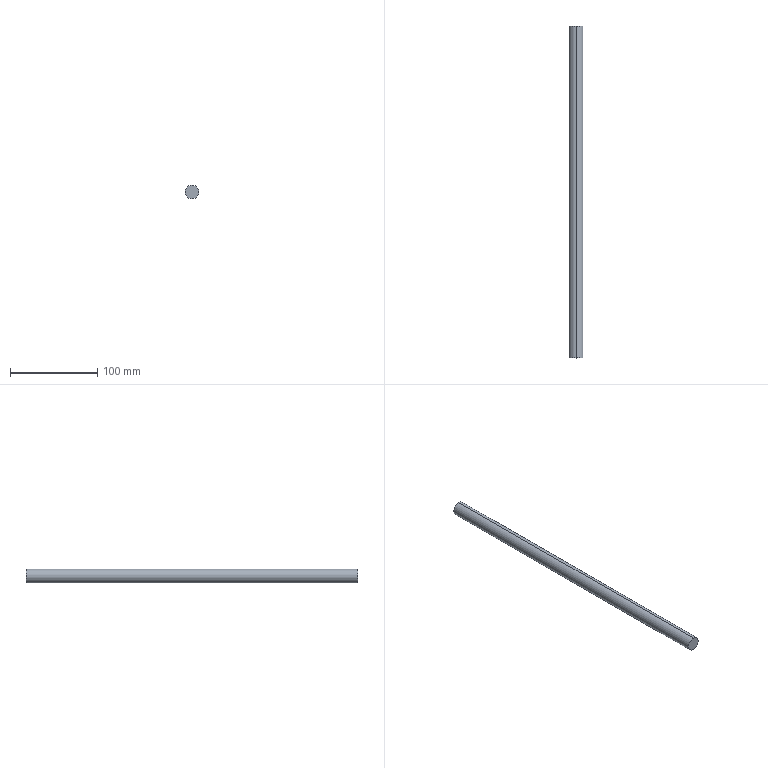Part | SolidWorks | features Extrusion 1 | 1 solid | 4 faces | box 16 x 380 x 16 mm | volume 76404 mm3 | cylinder 2 | plane 2 | commonest cylinder face diameters 16 x2
STEP:
#1=CARTESIAN_POINT('',(0.,380.,8.));
#2=VERTEX_POINT('',#1);
#3=CARTESIAN_POINT('',(0.,380.,-8.));
#4=VERTEX_POINT('',#3);
#5=CARTESIAN_POINT('',(0.,380.,0.));
#6=DIRECTION('',(0.,1.,0.));
#7=DIRECTION('',(0.,0.,1.));
#8=AXIS2_PLACEMENT_3D('',#5,#6,#7);
#9=CIRCLE('',#8,8.);
#10=EDGE_CURVE('',#2,#4,#9,.T.);
#11=ORIENTED_EDGE('',*,*,#10,.F.);
#12=CARTESIAN_POINT('',(0.,0.,8.));
#13=VERTEX_POINT('',#12);
#14=CARTESIAN_POINT('',(0.,380.,8.));
#15=DIRECTION('',(0.,-1.,0.));
#16=VECTOR('',#15,1000.);
#17=LINE('',#14,#16);
#18=EDGE_CURVE('',#2,#13,#17,.T.);
#19=ORIENTED_EDGE('',*,*,#18,.T.);
#20=CARTESIAN_POINT('',(0.,0.,-8.));
#21=VERTEX_POINT('',#20);
#22=CARTESIAN_POINT('',(0.,0.,0.));
#23=DIRECTION('',(0.,1.,0.));
#24=DIRECTION('',(0.,0.,1.));
#25=AXIS2_PLACEMENT_3D('',#22,#23,#24);
#26=CIRCLE('',#25,8.);
#27=EDGE_CURVE('',#13,#21,#26,.T.);
#28=ORIENTED_EDGE('',*,*,#27,.T.);
#29=CARTESIAN_POINT('',(0.,380.,-8.));
#30=DIRECTION('',(0.,-1.,0.));
#31=VECTOR('',#30,1000.);
#32=LINE('',#29,#31);
#33=EDGE_CURVE('',#4,#21,#32,.T.);
#34=ORIENTED_EDGE('',*,*,#33,.F.);
#35=EDGE_LOOP('',(#11,#19,#28,#34));
#36=FACE_OUTER_BOUND('',#35,.T.);
#37=CARTESIAN_POINT('',(0.,380.,0.));
#38=DIRECTION('',(0.,-1.,0.));
#39=DIRECTION('',(0.,0.,-1.));
#40=AXIS2_PLACEMENT_3D('',#37,#38,#39);
#41=CYLINDRICAL_SURFACE('',#40,8.);
#42=ADVANCED_FACE('',(#36),#41,.T.);
#43=ORIENTED_EDGE('',*,*,#18,.F.);
#44=CARTESIAN_POINT('',(0.,380.,0.));
#45=DIRECTION('',(0.,1.,0.));
#46=DIRECTION('',(0.,0.,1.));
#47=AXIS2_PLACEMENT_3D('',#44,#45,#46);
#48=CIRCLE('',#47,8.);
#49=EDGE_CURVE('',#4,#2,#48,.T.);
#50=ORIENTED_EDGE('',*,*,#49,.F.);
#51=ORIENTED_EDGE('',*,*,#33,.T.);
#52=CARTESIAN_POINT('',(0.,0.,0.));
#53=DIRECTION('',(0.,1.,0.));
#54=DIRECTION('',(0.,0.,1.));
#55=AXIS2_PLACEMENT_3D('',#52,#53,#54);
#56=CIRCLE('',#55,8.);
#57=EDGE_CURVE('',#21,#13,#56,.T.);
#58=ORIENTED_EDGE('',*,*,#57,.T.);
#59=EDGE_LOOP('',(#43,#50,#51,#58));
#60=FACE_OUTER_BOUND('',#59,.T.);
#61=CARTESIAN_POINT('',(0.,380.,0.));
#62=DIRECTION('',(0.,-1.,0.));
#63=DIRECTION('',(0.,0.,-1.));
#64=AXIS2_PLACEMENT_3D('',#61,#62,#63);
#65=CYLINDRICAL_SURFACE('',#64,8.);
#66=ADVANCED_FACE('',(#60),#65,.T.);
#67=ORIENTED_EDGE('',*,*,#49,.T.);
#68=ORIENTED_EDGE('',*,*,#10,.T.);
#69=EDGE_LOOP('',(#67,#68));
#70=FACE_OUTER_BOUND('',#69,.T.);
#71=CARTESIAN_POINT('',(0.,380.,0.));
#72=DIRECTION('',(0.,1.,0.));
#73=DIRECTION('',(0.,0.,1.));
#74=AXIS2_PLACEMENT_3D('',#71,#72,#73);
#75=PLANE('',#74);
#76=ADVANCED_FACE('',(#70),#75,.T.);
#77=ORIENTED_EDGE('',*,*,#57,.F.);
#78=ORIENTED_EDGE('',*,*,#27,.F.);
#79=EDGE_LOOP('',(#77,#78));
#80=FACE_OUTER_BOUND('',#79,.T.);
#81=CARTESIAN_POINT('',(0.,0.,0.));
#82=DIRECTION('',(0.,1.,0.));
#83=DIRECTION('',(0.,0.,1.));
#84=AXIS2_PLACEMENT_3D('',#81,#82,#83);
#85=PLANE('',#84);
#86=ADVANCED_FACE('',(#80),#85,.F.);
#87=CLOSED_SHELL('',(#42,#66,#76,#86));
#88=MANIFOLD_SOLID_BREP('',#87);
#89=CARTESIAN_POINT('',(0.,0.,0.));
#90=DIRECTION('',(0.,0.,1.));
#91=DIRECTION('',(1.,0.,0.));
#92=AXIS2_PLACEMENT_3D('',#89,#90,#91);
#93=(LENGTH_UNIT()NAMED_UNIT(*)SI_UNIT(.MILLI.,.METRE.));
#94=UNCERTAINTY_MEASURE_WITH_UNIT(LENGTH_MEASURE(0.00001),#93,'','');
#95=(NAMED_UNIT(*)PLANE_ANGLE_UNIT()SI_UNIT($,.RADIAN.));
#96=(NAMED_UNIT(*)SI_UNIT($,.STERADIAN.)SOLID_ANGLE_UNIT());
#97=(GEOMETRIC_REPRESENTATION_CONTEXT(3)GLOBAL_UNCERTAINTY_ASSIGNED_CONTEXT((#94))GLOBAL_UNIT_ASSIGNED_CONTEXT((#93,#95,#96))REPRESENTATION_CONTEXT('',''));
#98=ADVANCED_BREP_SHAPE_REPRESENTATION('',(#88,#92),#97);